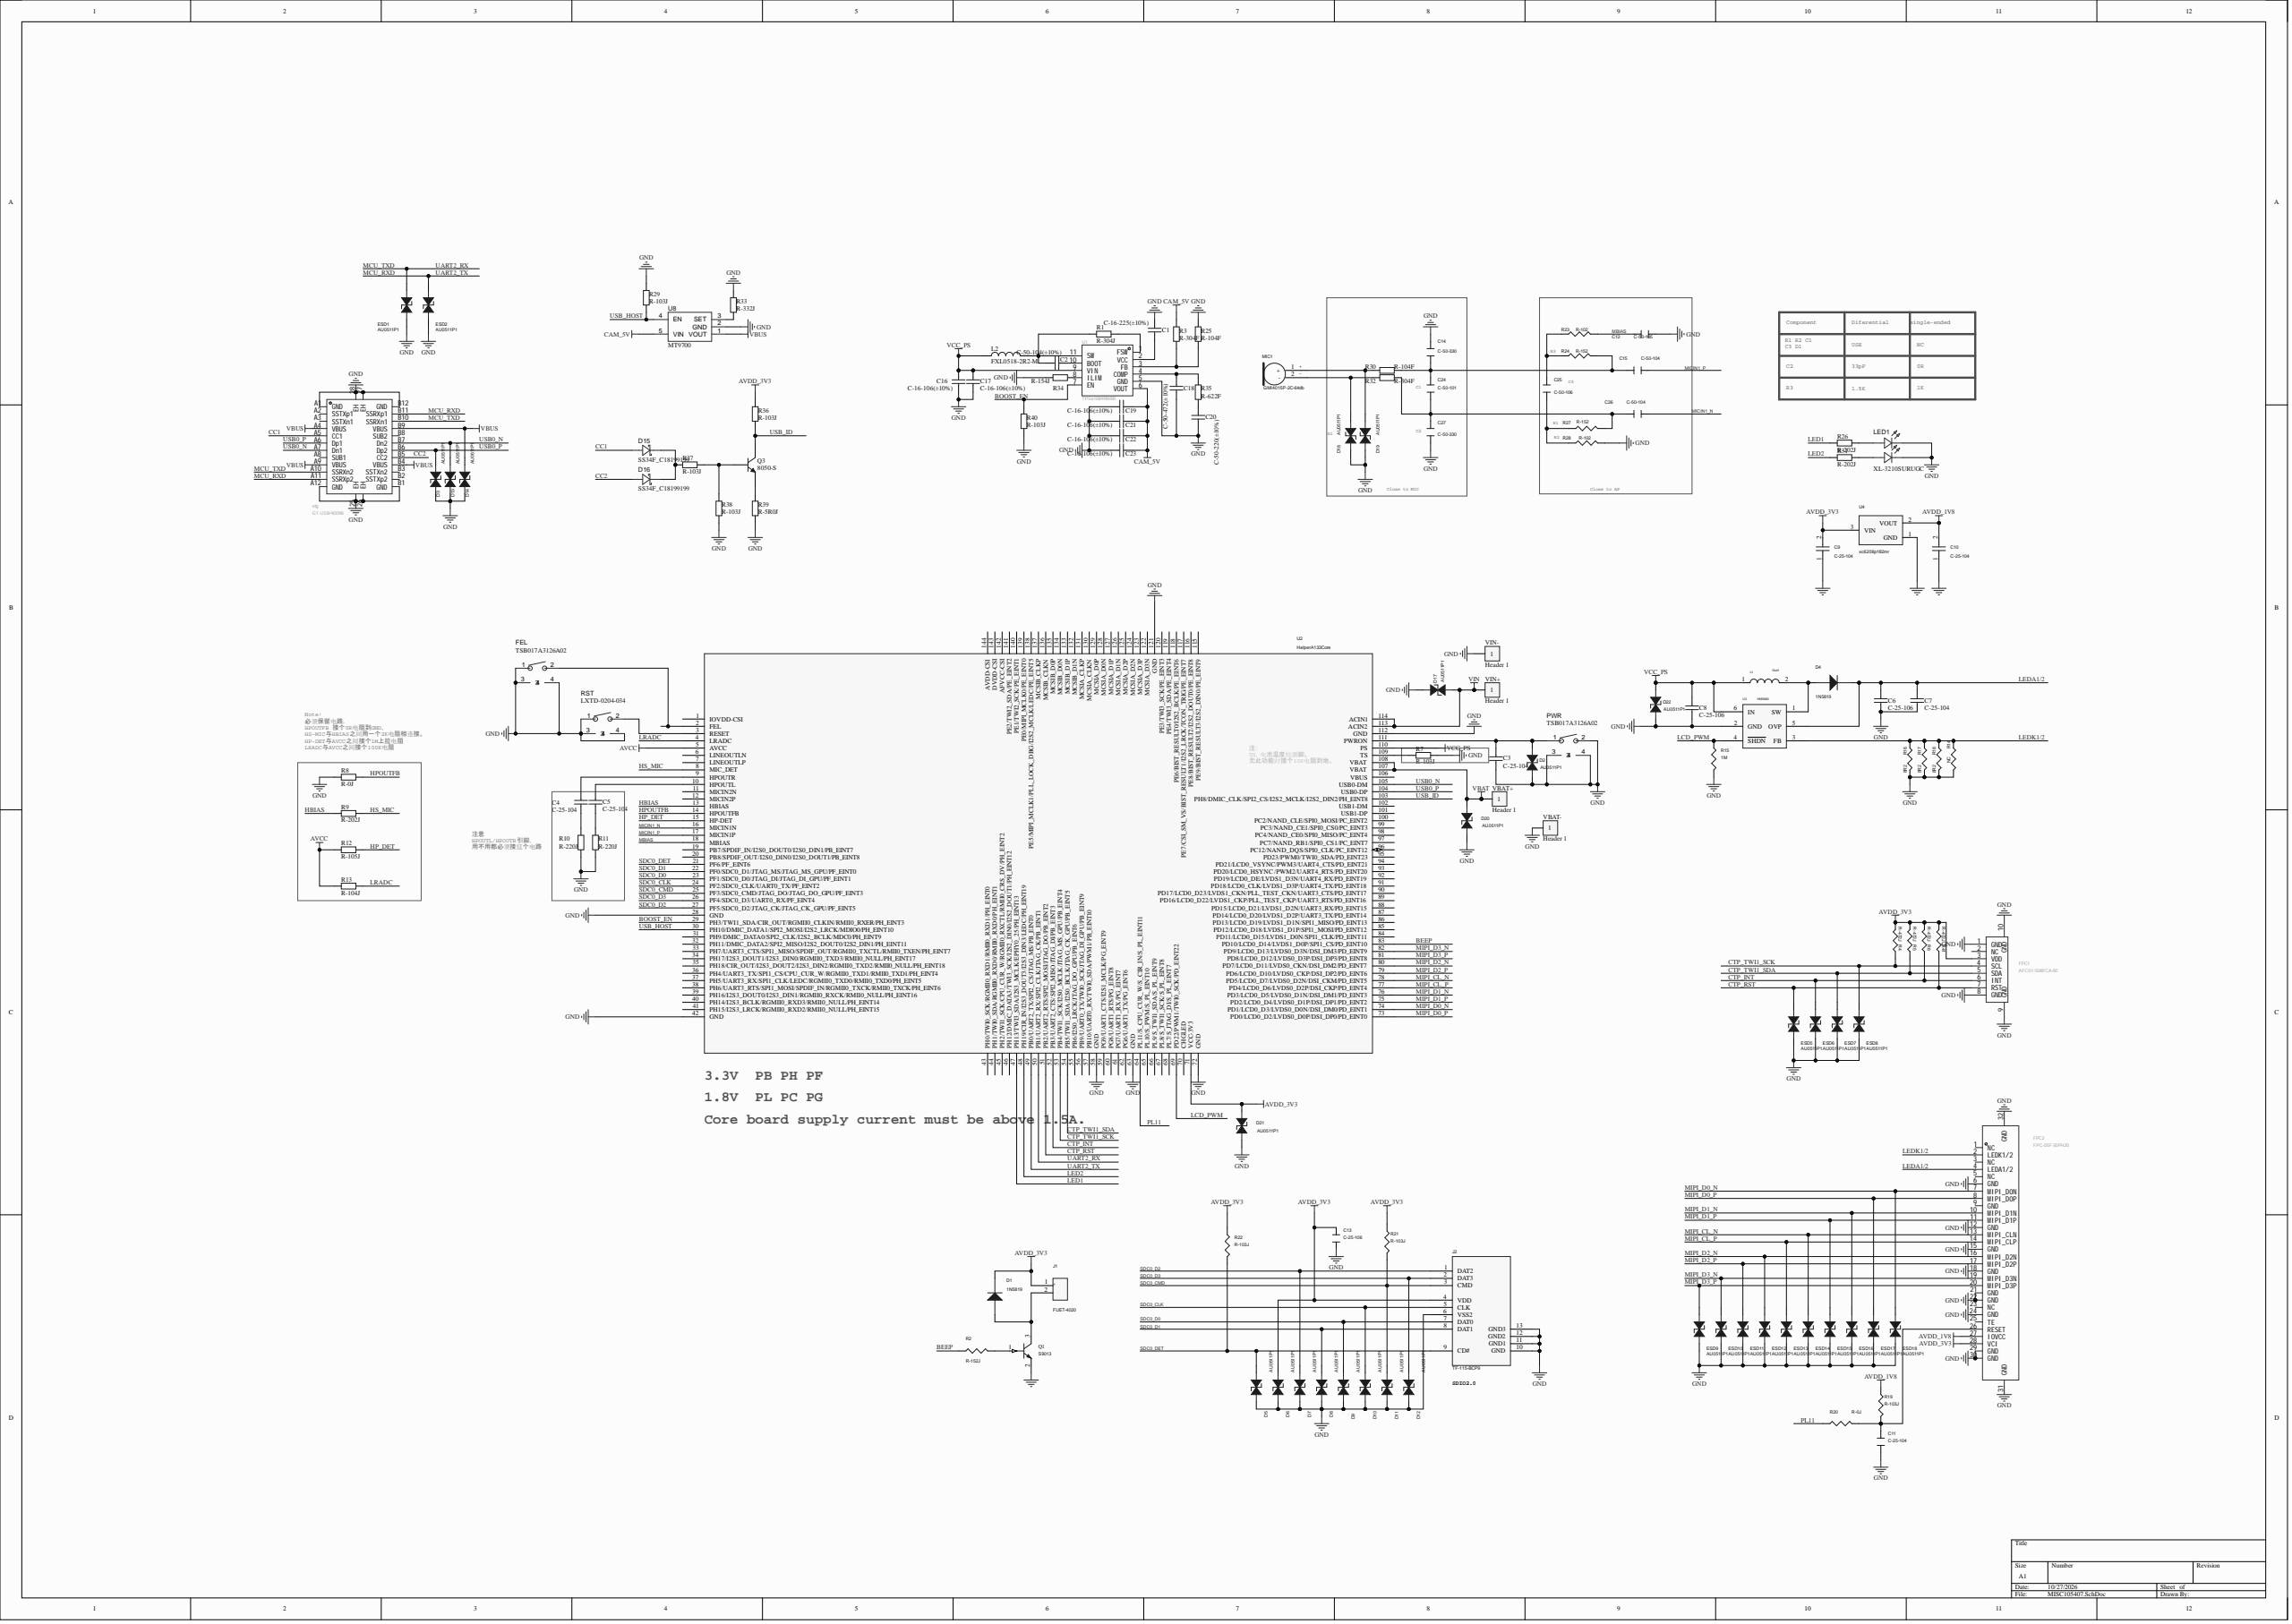Circuit board | Altium Designer | 129 parts | 86 nets
Bill of materials:
Comment,Description,Designator,Footprint,LibRef,Quantity
"C-16-225(±10%)","Chip capacitor","C1","C0402","C-XX-XXX","1"
"C-50-104(±10%)","Chip capacitor","C2","C0402","C-XX-XXX","1"
"C-25-104","Chip capacitor, [NoValue]","C3, C4, C5, C7, C9, C10, C11","C0402","C-XX-XXX, CAP NP_0, CAPACITOR_0","7"
"C-25-106","Chip capacitor, [NoValue]","C6, C8, C13","C0603","C-XX-XXX, CAPACITOR_0","3"
"C-50-105","","C12","C0402","C-C0402-X5R_0","1"
"C-50-330","","C14, C27","C0402","C-C0402-COG_0","2"
"C-50-104","","C15, C26","C0402","C-C0402-X5R_0","2"
"C-16-106(±10%)","Chip capacitor","C16, C17, C19, C21, C22, C23","C0603","C-XX-XXX","6"
"C-50-472(±10%)","Chip capacitor","C18","C0402","C-XX-XXX","1"
"C-50-220(±10%)","Chip capacitor","C20","C0402","C-XX-XXX","1"
"C-50-101","","C24","C0402","C-C0402-X5R_0","1"
"C-50-106","","C25","C0603","C-C0603-X5R_1","1"
"1N5819","","D1, D4","SOD323","BAS21/SOT_1","2"
"AU0511P1","","D2, D3, D5, D6, D7, D8, D9, D10, D11, D12, D13, D14, D17, D18, D19, D20, D21, D22, ESD1, ESD2, ESD5, ESD6, ESD7, ESD8, ESD9, ESD10, ESD11, ESD12, ESD13, ESD14, ESD15, ESD16, ESD17, ESD18","ESD0402A","1_1.5KE100A, ESD9B5VL","34"
"SS34F_C18199199","","D15, D16","SMAF_L3.5-W2.6-LS4.7-RD-1","SS34F_C18199199","2"
"TSB017A3126A02","","FEL, PWR","KEY-SMD_YTSB017A0312502B","TSB017A3126A02","2"
"AFC01-S08FCA-00","","FPC1","FPC-SMD_P0.50-8P_FGS-XJ-H2.0","FPC-05F-8PH20","1"
"FPC-05F-30PH20","","FPC2","FPC-SMD_30P-P0.50_XUNPU_FPC-05F-30PH20","FPC-05F-30PH20","1"
"FUET-4020","","J1","BUZ-SMD_L4.0-W4.0-P3.50-L","CON2_0","1"
"TF-115-BCP9","","J2","TF-SMD_TF-115-BCP9","SDMMC SLOT_0","1"
"10uH","","L1","IND-SMD_L2.5-W2.0","INDUCTOR","1"
"FXL0518-2R2-M","Low-power chip inductor","L2","IND-SMD_L5.2-W5.4","L","1"
"XL-3210SURUGC","","LED1","LED-SMD_4P-L3.2-W1.5_HTG-3210SURUBGC","XL-3210SURUGC","1"
"GMI4015P-2C-64db","","MIC1","MIC-TH_BD4.0-P1.40-D0.4-L-FD","Micphone_0","1"
"GT-USB-9009B","","otg","USB-C-SMD_GT-USB-9009B","TYPE-C-31-M-01","1"
"S9013","","Q1","SOT23","2N3904_0","1"
"8050-S","NPN transistor","Q3","SOT-23-3","8050-S","1"
"R-304J","Chip resistor","R1","R0402","R-XXXJ","1"
"R-152J","","R2","R0402","R_Dup2","1"
"R-304F","Chip resistor","R3, R32","R0402","R-XXXJ","2"
"R-472J","","R4, R5, R6, R41","R0402","R","4"
"R-103J","Chip resistor, [NoValue]","R7, R19, R21, R22, R29, R36, R37, R38, R40","R0402","R-XXXJ, R_Dup7","9"
"R-0J","Chip resistor, [NoValue]","R8, R20","R0402","R-XXXJ, R","2"
"R-202J","Chip resistor","R9, R26, R31","R0402","R-XXXJ","3"
"R-220J","Chip resistor","R10, R11","R0402","R-XXXJ","2"
"R-105J","Chip resistor","R12","R0402","R-XXXJ","1"
"R-104J","Chip resistor","R13","R0402","R-XXXJ","1"
"NC","","R14","R0402","R","1"
"1M","","R15","R0402","R","1"
"8R2","","R16, R17, R18","R0402","R","3"
"R-102","","R23, R28","R0402","R-R0402-5%_Dup1","2"
"R-152","","R24, R27","R0402","R-R0402-5%_Dup1","2"
"R-104F","Chip resistor","R25, R30","R0402","R-XXXJ","2"
"R-332J","Chip resistor","R33","R0402","R-XXXJ","1"
"R-154J","Chip resistor","R34","R0402","R-XXXJ","1"
"R-622F","Chip resistor","R35","R0402","R-XXXJ","1"
"R-5R0J","Chip resistor","R39","R0402","R-XXXJ","1"
"LXTD-0204-034","","RST","SW-SMD_LXTD-0204-034","TSB017A3126A02","1"
"TPS61089RNRR","","U1","VQFN-HR_L2.5-W2.0-P0.50-TL-EP","TPS61089RNRR","1"
"HelperA133Core","","U2","A133","SOC2416_8","1"
"HM5663","","U3","SOT23-6","PT4110_0","1"
"xc6206p182mr","","U4","SOT23","SGM2028_0","1"
"MT9700","","U8","SOT-23-5_L3.0-W1.7-P0.95-LS2.8-BR","MT9700","1"
"Header 1","1P","VBAT-, VBAT+, VIN-, VIN+","HDR-LI-1P","Header 1","4"
Netlist (Protel format):
[
C1
C0402
C-16-225(±10%)



]
[
C2
C0402
C-50-104(±10%)



]
[
C3
C0402
C-25-104



]
[
C4
C0402
C-25-104



]
[
C5
C0402
C-25-104



]
[
C6
C0603
C-25-106



]
[
C7
C0402
C-25-104



]
[
C8
C0603
C-25-106



]
[
C9
C0402
C-25-104



]
[
C10
C0402
C-25-104



]
[
C11
C0402
C-25-104



]
[
C12
C0402
C-50-105



]
[
C13
C0603
C-25-106



]
[
C14
C0402
C-50-330



]
[
C15
C0402
C-50-104



]
[
C16
C0603
C-16-106(±10%)



]
[
C17
C0603
C-16-106(±10%)



]
[
C18
C0402
C-50-472(±10%)



]
[
C19
C0603
C-16-106(±10%)



]
[
C20
C0402
C-50-220(±10%)



]
[
C21
C0603
C-16-106(±10%)



]
[
C22
C0603
C-16-106(±10%)



]
[
C23
C0603
C-16-106(±10%)



]
[
C24
C0402
C-50-101



]
[
C25
C0603
C-50-106



]
[
C26
C0402
C-50-104



]
[
C27
C0402
C-50-330



]
[
D1
SOD323
1N5819



]
[
D2
ESD0402A
AU0511P1



]
[
D3
ESD0402A
AU0511P1



]
[
D4
SOD323
1N5819



]
[
D5
ESD0402A
AU0511P1



]
[
D6
ESD0402A
AU0511P1



]
[
D7
ESD0402A
AU0511P1



]
[
D8
ESD0402A
AU0511P1



]
[
D9
ESD0402A
AU0511P1



]
[
D10
ESD0402A
AU0511P1



]
[
D11
ESD0402A
AU0511P1



]
[
D12
ESD0402A
AU0511P1



]
[
D13
ESD0402A
AU0511P1



]
[
D14
ESD0402A
AU0511P1



]
[
D15
SMAF_L3.5-W2.6-LS4.7-RD-1
SS34F_C18199199



]
[
D16
SMAF_L3.5-W2.6-LS4.7-RD-1
SS34F_C18199199



]
[
D17
ESD0402A
AU0511P1



]
[
D18
ESD0402A
AU0511P1



]
[
D19
ESD0402A
AU0511P1



]
[
D20
ESD0402A
AU0511P1



]
[
D21
ESD0402A
AU0511P1



]
[
D22
ESD0402A
AU0511P1



]
[
ESD1
ESD0402A
AU0511P1



]
[
ESD2
ESD0402A
AU0511P1



]
[
ESD5
ESD0402A
AU0511P1



]
[
ESD6
ESD0402A
AU0511P1



]
[
ESD7
ESD0402A
AU0511P1



]
[
ESD8
ESD0402A
AU0511P1



]
[
ESD9
ESD0402A
AU0511P1



]
[
ESD10
ESD0402A
AU0511P1



]
[
ESD11
ESD0402A
AU0511P1



]
[
ESD12
ESD0402A
AU0511P1



]
[
ESD13
ESD0402A
AU0511P1



]
[
ESD14
ESD0402A
AU0511P1



]
[
ESD15
ESD0402A
AU0511P1



]
[
ESD16
ESD0402A
AU0511P1



]
[
ESD17
ESD0402A
AU0511P1



]
[
ESD18
ESD0402A
AU0511P1



]
[
FEL
KEY-SMD_YTSB017A0312502B
TSB017A3126A02



]
[
FPC1
FPC-SMD_P0.50-8P_FGS-XJ-H2.0
AFC01-S08FCA-00



]
[
FPC2
FPC-SMD_30P-P0.50_XUNPU_FPC-05F-30PH20
FPC-05F-30PH20



]
[
J1
BUZ-SMD_L4.0-W4.0-P3.50-L
FUET-4020



]
[
J2
TF-SMD_TF-115-BCP9
TF-115-BCP9



]
[
L1
IND-SMD_L2.5-W2.0
10uH



]
[
L2
IND-SMD_L5.2-W5.4
FXL0518-2R2-M



]
[
LED1
LED-SMD_4P-L3.2-W1.5_HTG-3210SURUBGC
XL-3210SURUGC



]
[
MIC1
MIC-TH_BD4.0-P1.40-D0.4-L-FD
GMI4015P-2C-64db



]
[
otg
USB-C-SMD_GT-USB-9009B
GT-USB-9009B



]
[
PWR
KEY-SMD_YTSB017A0312502B
TSB017A3126A02



]
[
Q1
SOT23
S9013



]
[
Q3
SOT-23-3
8050-S



]
[
R1
R0402
R-304J



]
[
R2
R0402
R-152J



]
[
R3
R0402
R-304F



]
[
R4
R0402
R-472J



]
[
R5
R0402
R-472J



]
[
R6
R0402
R-472J



]
[
R7
R0402
R-103J



]
[
R8
R0402
R-0J



]
[
R9
R0402
R-202J



]
[
R10
R0402
R-220J



]
[
R11
R0402
R-220J



]
[
R12
R0402
R-105J



]
[
R13
R0402
R-104J



]
[
R14
R0402
NC



]
[
R15
R0402
1M



]
[
R16
R0402
8R2



]
[
R17
R0402
8R2



]
[
R18
R0402
8R2



]
[
R19
R0402
R-103J



]
[
R20
R0402
R-0J



]
[
R21
R0402
R-103J



]
[
R22
R0402
R-103J



]
[
R23
R0402
R-102



]
[
R24
R0402
R-152



]
[
R25
R0402
R-104F



]
[
R26
R0402
R-202J



]
[
R27
R0402
R-152



]
[
R28
R0402
R-102



]
[
R29
R0402
R-103J



]
[
R30
R0402
R-104F



]
[
R31
R0402
R-202J



]
[
R32
R0402
R-304F



]
[
R33
R0402
R-332J



]
[
R34
R0402
R-154J



]
[
R35
R0402
R-622F



]
[
R36
R0402
R-103J



]
[
R37
R0402
R-103J



]
[
R38
R0402
R-103J



]
[
R39
R0402
R-5R0J



]
[
R40
R0402
R-103J



]
[
R41
R0402
R-472J



]
[
RST
SW-SMD_LXTD-0204-034
LXTD-0204-034



]
[
U1
VQFN-HR_L2.5-W2.0-P0.50-TL-EP
TPS61089RNRR



]
[
U2
A133
HelperA133Core



]
[
U3
SOT23-6
HM5663



]
[
U4
SOT23
xc6206p182mr



]
[
U8
SOT-23-5_L3.0-W1.7-P0.95-LS2.8-BR
MT9700



]
[
VBAT+
HDR-LI-1P
Header 1



]
[
VBAT-
HDR-LI-1P
Header 1



]
[
VIN+
HDR-LI-1P
Header 1



]
[
VIN-
HDR-LI-1P
Header 1



]
(
VIN
D17-1
U2-113
U2-114
VIN+-1
)
(
VCC_PS
C8-1
C16-2
C17-2
D22-2
L1-1
L2-1
U1-9
U2-110
U3-6
)
(
VBUS
D14-1
otg-A4
otg-A9
otg-B4
otg-B9
U8-1
)
(
VBAT
D20-1
U2-107
U2-108
VBAT+-1
)
(
USB_ID
Q3-3
R36-2
U2-103
)
(
USB_HOST
R29-1
U2-30
U8-4
)
(
USB0_P
D3-1
otg-A6
otg-B6
U2-104
)
(
USB0_N
D13-1
otg-A7
otg-B7
U2-105
)
(
SDC0_DET
D5-1
J2-9
R22-2
U2-21
)
(
SDC0_D3
D12-1
J2-2
U2-26
)
(
SDC0_D2
D7-1
J2-1
U2-27
)
(
SDC0_D1
D8-1
J2-8
U2-22
)
(
SDC0_D0
D9-1
J2-7
U2-23
)
(
SDC0_CMD
D11-1
J2-3
R21-2
U2-25
)
(
SDC0_CLK
D10-1
J2-5
U2-24
)
(
PL11
R20-1
U2-64
)
(
NetRST_2
RST-2
U2-3
)
(
NetR34_2
R34-2
U1-8
)
(
NetR33_1
R33-1
U8-3
)
(
NetR7_2
R7-2
U2-109
)
(
NetR3_1
R3-1
R25-1
U1-3
)
(
NetR1_2
R1-2
U1-1
)
(
NetQ3_2
Q3-2
R39-1
)
(
NetQ3_1
Q3-1
R37-1
R38-1
)
(
NetQ1_1
Q1-1
R2-2
)
(
NetLED1_3
LED1-3
R31-2
)
(
NetLED1_1
LED1-1
R26-2
)
(
NetFEL_2
FEL-2
U2-2
)
(
NetD19_2
D19-2
MIC1-1
R30-2
)
(
NetD18_2
D18-2
MIC1-2
R32-2
)
(
NetD15_1
D15-1
D16-1
R37-2
)
(
NetD4_1
D4-1
L1-2
U3-1
)
(
NetD1_1
D1-1
J1-2
Q1-3
)
(
NetC25_2
C25-2
R27-1
R28-1
)
(
NetC25_1
C25-1
R23-1
R24-1
)
(
NetC24_2
C24-2
C26-1
C27-1
R27-2
R32-1
)
(
NetC20_1
C20-1
R35-2
)
(
NetC18_1
C18-1
R35-1
U1-4
)
(
NetC14_1
C14-1
C15-1
C24-1
R24-2
R30-1
)
(
NetC11_2
C11-2
FPC2-26
R19-2
R20-2
)
(
NetC5_2
C5-2
R11-2
)
(
NetC5_1
C5-1
U2-10
)
(
NetC4_2
C4-2
R10-1
)
(
NetC4_1
C4-1
U2-9
)
(
NetC3_1
C3-1
D2-2
PWR-1
U2-111
)
(
NetC2_2
C2-2
L2-2
R1-1
U1-11
)
(
NetC2_1
C2-1
U1-10
)
(
NetC1_2
C1-2
U1-2
)
(
MIPI_D3_P
ESD9-1
FPC2-20
U2-81
)
(
MIPI_D3_N
ESD10-1
FPC2-19
U2-82
)
(
MIPI_D2_P
ESD11-1
FPC2-17
U2-79
)
(
MIPI_D2_N
ESD12-1
FPC2-16
U2-80
)
(
MIPI_D1_P
ESD15-1
FPC2-11
U2-75
)
(
MIPI_D1_N
ESD16-1
FPC2-10
U2-76
)
(
MIPI_D0_P
ESD17-1
FPC2-8
U2-73
)
(
MIPI_D0_N
ESD18-1
FPC2-7
U2-74
)
(
MIPI_CL_P
ESD13-1
FPC2-14
U2-77
)
(
MIPI_CL_N
ESD14-1
FPC2-13
U2-78
)
(
MICIN1_P
C15-2
U2-17
)
(
MICIN1_N
C26-2
U2-16
)
(
MCU_TXD
ESD1-1
otg-A10
otg-B10
U2-50
)
(
MCU_RXD
ESD2-1
otg-A11
otg-B11
U2-49
)
(
MBIAS
C12-1
R23-2
U2-18
)
(
LRADC
R13-2
U2-4
)
(
LEDK1/2
FPC2-2
R14-1
R16-1
R17-1
R18-1
U3-3
)
(
LEDA1/2
C6-1
C7-1
D4-2
FPC2-4
U3-5
)
(
LED2
R31-1
U2-48
)
(
LED1
R26-1
U2-47
)
(
LCD_PWM
R15-1
U2-69
U3-4
)
(
HS_MIC
R9-2
U2-8
)
(
HPOUTFB
R8-2
U2-14
)
(
HP_DET
R12-2
U2-15
)
(
HBIAS
R9-1
U2-13
)
(
GND
C1-1
C3-2
C6-2
C7-2
C8-2
C9-1
C10-1
C11-1
C12-2
C13-1
C14-2
C16-1
C17-1
C18-2
C19-1
C20-2
C21-1
C22-1
C23-1
C27-2
D2-1
D3-2
D5-2
D6-2
D7-2
D8-2
D9-2
D10-2
D11-2
D12-2
D13-2
D14-2
D17-2
D18-1
D19-1
D20-2
D21-2
D22-1
ESD1-2
ESD2-2
ESD5-2
ESD6-2
ESD7-2
ESD8-2
ESD9-2
ESD10-2
ESD11-2
ESD12-2
ESD13-2
ESD14-2
ESD15-2
ESD16-2
ESD17-2
ESD18-2
FEL-1
FEL-3
FEL-4
FPC1-1
FPC1-8
FPC1-9
FPC1-10
FPC2-6
FPC2-12
FPC2-15
FPC2-18
FPC2-21
FPC2-22
FPC2-24
FPC2-29
FPC2-30
FPC2-31
FPC2-32
J2-6
J2-10
J2-11
J2-12
J2-13
LED1-2
LED1-4
otg-25
otg-26
otg-27
otg-28
otg-A1
otg-A12
otg-B1
otg-B12
PWR-2
PWR-3
PWR-4
Q1-2
R7-1
R8-1
R10-2
R11-1
R14-2
R15-2
R16-2
R17-2
R18-2
R25-2
R28-2
R29-2
R33-2
R34-1
R38-2
R39-2
R40-2
RST-1
RST-3
RST-4
U1-5
U2-28
U2-42
U2-58
U2-63
U2-72
U2-112
U2-121
U3-2
U4-1
U8-2
VBAT--1
VIN--1
)
(
CTP_TWI1_SDA
ESD7-1
FPC1-5
R5-1
U2-54
)
(
CTP_TWI1_SCK
ESD8-1
FPC1-4
R4-1
U2-53
)
(
CTP_RST
ESD5-1
FPC1-7
R41-1
U2-51
)
(
CTP_INT
ESD6-1
FPC1-6
R6-1
U2-52
)
(
CC2
D16-2
otg-B5
)
(
CC1
D15-2
otg-A5
)
(
CAM_5V
C19-2
C21-2
C22-2
C23-2
R3-2
U1-6
U8-5
)
(
BOOST_EN
R40-1
U1-7
U2-29
)
(
BEEP
R2-1
U2-83
)
(
AVDD_3V3
C9-2
C13-2
D1-2
D6-1
D21-1
FPC1-3
FPC2-28
J1-1
J2-4
R4-2
R5-2
R6-2
R21-1
R22-1
R36-1
R41-2
U2-71
U4-3
)
(
AVDD_1V8
C10-2
FPC2-27
R19-1
U4-2
)
(
AVCC
R12-1
R13-1
U2-5
)